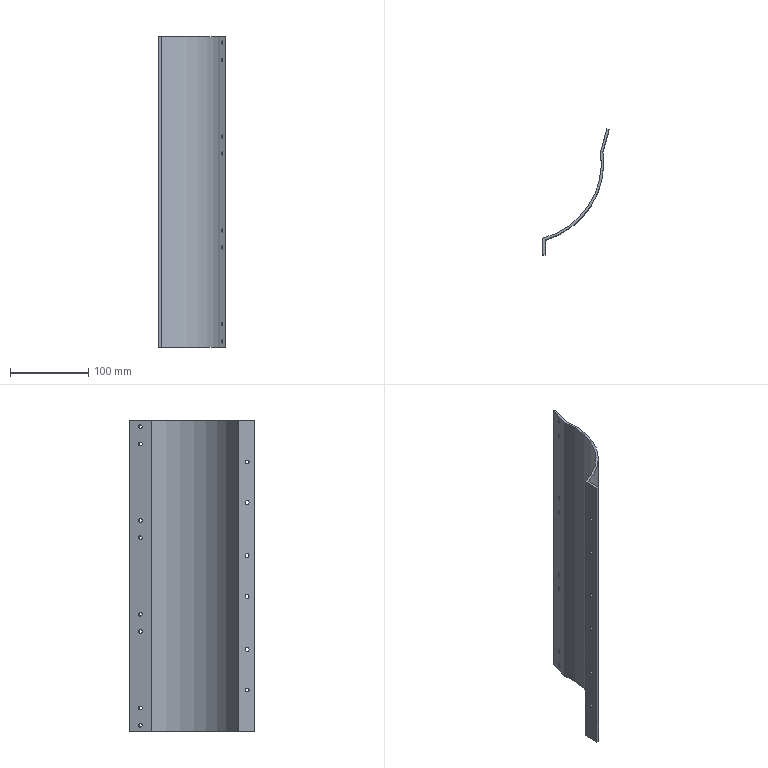Part | SolidWorks | features BaseBody 1 | 1 solid | 38 faces | box 85.064 x 161.136 x 398 mm | volume 233857 mm3 | cylinder 30 | plane 8 | commonest cylinder face diameters 5 x28 200 x1 206 x1
STEP:
#1=CARTESIAN_POINT('',(103.077,28.708,-32.5));
#2=VERTEX_POINT('',#1);
#3=CARTESIAN_POINT('',(103.077,28.708,-27.5));
#4=VERTEX_POINT('',#3);
#5=CARTESIAN_POINT('',(103.077,28.708,-30.));
#6=DIRECTION('',(0.9619,-0.2734,0.));
#7=DIRECTION('',(0.,0.,1.));
#8=AXIS2_PLACEMENT_3D('',#5,#6,#7);
#9=CIRCLE('',#8,2.5);
#10=EDGE_CURVE('',#2,#4,#9,.T.);
#11=ORIENTED_EDGE('',*,*,#10,.F.);
#12=CARTESIAN_POINT('',(105.962,27.888,-32.5));
#13=VERTEX_POINT('',#12);
#14=CARTESIAN_POINT('',(105.962,27.888,-32.5));
#15=DIRECTION('',(0.9619,-0.2734,0.));
#16=VECTOR('',#15,1000.);
#17=LINE('',#14,#16);
#18=EDGE_CURVE('',#2,#13,#17,.T.);
#19=ORIENTED_EDGE('',*,*,#18,.T.);
#20=CARTESIAN_POINT('',(105.962,27.888,-27.5));
#21=VERTEX_POINT('',#20);
#22=CARTESIAN_POINT('',(105.962,27.888,-30.));
#23=DIRECTION('',(-0.9619,0.2734,0.));
#24=DIRECTION('',(0.,0.,1.));
#25=AXIS2_PLACEMENT_3D('',#22,#23,#24);
#26=CIRCLE('',#25,2.5);
#27=EDGE_CURVE('',#21,#13,#26,.T.);
#28=ORIENTED_EDGE('',*,*,#27,.F.);
#29=CARTESIAN_POINT('',(105.962,27.888,-27.5));
#30=DIRECTION('',(0.9619,-0.2734,0.));
#31=VECTOR('',#30,1000.);
#32=LINE('',#29,#31);
#33=EDGE_CURVE('',#4,#21,#32,.T.);
#34=ORIENTED_EDGE('',*,*,#33,.F.);
#35=EDGE_LOOP('',(#11,#19,#28,#34));
#36=FACE_OUTER_BOUND('',#35,.T.);
#37=CARTESIAN_POINT('',(105.962,27.888,-30.));
#38=DIRECTION('',(0.9619,-0.2734,0.));
#39=DIRECTION('',(0.,0.,1.));
#40=AXIS2_PLACEMENT_3D('',#37,#38,#39);
#41=CYLINDRICAL_SURFACE('',#40,2.5);
#42=ADVANCED_FACE('',(#36),#41,.F.);
#43=CARTESIAN_POINT('',(103.077,28.708,-10.5));
#44=VERTEX_POINT('',#43);
#45=CARTESIAN_POINT('',(103.077,28.708,-5.5));
#46=VERTEX_POINT('',#45);
#47=CARTESIAN_POINT('',(103.077,28.708,-8.));
#48=DIRECTION('',(0.9619,-0.2734,0.));
#49=DIRECTION('',(0.,0.,1.));
#50=AXIS2_PLACEMENT_3D('',#47,#48,#49);
#51=CIRCLE('',#50,2.5);
#52=EDGE_CURVE('',#44,#46,#51,.T.);
#53=ORIENTED_EDGE('',*,*,#52,.F.);
#54=CARTESIAN_POINT('',(105.962,27.888,-10.5));
#55=VERTEX_POINT('',#54);
#56=CARTESIAN_POINT('',(105.962,27.888,-10.5));
#57=DIRECTION('',(0.9619,-0.2734,0.));
#58=VECTOR('',#57,1000.);
#59=LINE('',#56,#58);
#60=EDGE_CURVE('',#44,#55,#59,.T.);
#61=ORIENTED_EDGE('',*,*,#60,.T.);
#62=CARTESIAN_POINT('',(105.962,27.888,-5.5));
#63=VERTEX_POINT('',#62);
#64=CARTESIAN_POINT('',(105.962,27.888,-8.));
#65=DIRECTION('',(-0.9619,0.2734,0.));
#66=DIRECTION('',(0.,0.,1.));
#67=AXIS2_PLACEMENT_3D('',#64,#65,#66);
#68=CIRCLE('',#67,2.5);
#69=EDGE_CURVE('',#63,#55,#68,.T.);
#70=ORIENTED_EDGE('',*,*,#69,.F.);
#71=CARTESIAN_POINT('',(105.962,27.888,-5.5));
#72=DIRECTION('',(0.9619,-0.2734,0.));
#73=VECTOR('',#72,1000.);
#74=LINE('',#71,#73);
#75=EDGE_CURVE('',#46,#63,#74,.T.);
#76=ORIENTED_EDGE('',*,*,#75,.F.);
#77=EDGE_LOOP('',(#53,#61,#70,#76));
#78=FACE_OUTER_BOUND('',#77,.T.);
#79=CARTESIAN_POINT('',(105.962,27.888,-8.));
#80=DIRECTION('',(0.9619,-0.2734,0.));
#81=DIRECTION('',(0.,0.,1.));
#82=AXIS2_PLACEMENT_3D('',#79,#80,#81);
#83=CYLINDRICAL_SURFACE('',#82,2.5);
#84=ADVANCED_FACE('',(#78),#83,.F.);
#85=CARTESIAN_POINT('',(103.077,28.708,-152.5));
#86=VERTEX_POINT('',#85);
#87=CARTESIAN_POINT('',(103.077,28.708,-147.5));
#88=VERTEX_POINT('',#87);
#89=CARTESIAN_POINT('',(103.077,28.708,-150.));
#90=DIRECTION('',(0.9619,-0.2734,0.));
#91=DIRECTION('',(0.,0.,1.));
#92=AXIS2_PLACEMENT_3D('',#89,#90,#91);
#93=CIRCLE('',#92,2.5);
#94=EDGE_CURVE('',#86,#88,#93,.T.);
#95=ORIENTED_EDGE('',*,*,#94,.F.);
#96=CARTESIAN_POINT('',(105.962,27.888,-152.5));
#97=VERTEX_POINT('',#96);
#98=CARTESIAN_POINT('',(105.962,27.888,-152.5));
#99=DIRECTION('',(0.9619,-0.2734,0.));
#100=VECTOR('',#99,1000.);
#101=LINE('',#98,#100);
#102=EDGE_CURVE('',#86,#97,#101,.T.);
#103=ORIENTED_EDGE('',*,*,#102,.T.);
#104=CARTESIAN_POINT('',(105.962,27.888,-147.5));
#105=VERTEX_POINT('',#104);
#106=CARTESIAN_POINT('',(105.962,27.888,-150.));
#107=DIRECTION('',(-0.9619,0.2734,0.));
#108=DIRECTION('',(0.,0.,1.));
#109=AXIS2_PLACEMENT_3D('',#106,#107,#108);
#110=CIRCLE('',#109,2.5);
#111=EDGE_CURVE('',#105,#97,#110,.T.);
#112=ORIENTED_EDGE('',*,*,#111,.F.);
#113=CARTESIAN_POINT('',(105.962,27.888,-147.5));
#114=DIRECTION('',(0.9619,-0.2734,0.));
#115=VECTOR('',#114,1000.);
#116=LINE('',#113,#115);
#117=EDGE_CURVE('',#88,#105,#116,.T.);
#118=ORIENTED_EDGE('',*,*,#117,.F.);
#119=EDGE_LOOP('',(#95,#103,#112,#118));
#120=FACE_OUTER_BOUND('',#119,.T.);
#121=CARTESIAN_POINT('',(105.962,27.888,-150.));
#122=DIRECTION('',(0.9619,-0.2734,0.));
#123=DIRECTION('',(0.,0.,1.));
#124=AXIS2_PLACEMENT_3D('',#121,#122,#123);
#125=CYLINDRICAL_SURFACE('',#124,2.5);
#126=ADVANCED_FACE('',(#120),#125,.F.);
#127=CARTESIAN_POINT('',(103.077,28.708,-130.5));
#128=VERTEX_POINT('',#127);
#129=CARTESIAN_POINT('',(103.077,28.708,-125.5));
#130=VERTEX_POINT('',#129);
#131=CARTESIAN_POINT('',(103.077,28.708,-128.));
#132=DIRECTION('',(0.9619,-0.2734,0.));
#133=DIRECTION('',(0.,0.,1.));
#134=AXIS2_PLACEMENT_3D('',#131,#132,#133);
#135=CIRCLE('',#134,2.5);
#136=EDGE_CURVE('',#128,#130,#135,.T.);
#137=ORIENTED_EDGE('',*,*,#136,.F.);
#138=CARTESIAN_POINT('',(105.962,27.888,-130.5));
#139=VERTEX_POINT('',#138);
#140=CARTESIAN_POINT('',(105.962,27.888,-130.5));
#141=DIRECTION('',(0.9619,-0.2734,0.));
#142=VECTOR('',#141,1000.);
#143=LINE('',#140,#142);
#144=EDGE_CURVE('',#128,#139,#143,.T.);
#145=ORIENTED_EDGE('',*,*,#144,.T.);
#146=CARTESIAN_POINT('',(105.962,27.888,-125.5));
#147=VERTEX_POINT('',#146);
#148=CARTESIAN_POINT('',(105.962,27.888,-128.));
#149=DIRECTION('',(-0.9619,0.2734,0.));
#150=DIRECTION('',(0.,0.,1.));
#151=AXIS2_PLACEMENT_3D('',#148,#149,#150);
#152=CIRCLE('',#151,2.5);
#153=EDGE_CURVE('',#147,#139,#152,.T.);
#154=ORIENTED_EDGE('',*,*,#153,.F.);
#155=CARTESIAN_POINT('',(105.962,27.888,-125.5));
#156=DIRECTION('',(0.9619,-0.2734,0.));
#157=VECTOR('',#156,1000.);
#158=LINE('',#155,#157);
#159=EDGE_CURVE('',#130,#147,#158,.T.);
#160=ORIENTED_EDGE('',*,*,#159,.F.);
#161=EDGE_LOOP('',(#137,#145,#154,#160));
#162=FACE_OUTER_BOUND('',#161,.T.);
#163=CARTESIAN_POINT('',(105.962,27.888,-128.));
#164=DIRECTION('',(0.9619,-0.2734,0.));
#165=DIRECTION('',(0.,0.,1.));
#166=AXIS2_PLACEMENT_3D('',#163,#164,#165);
#167=CYLINDRICAL_SURFACE('',#166,2.5);
#168=ADVANCED_FACE('',(#162),#167,.F.);
#169=CARTESIAN_POINT('',(103.077,28.708,-272.5));
#170=VERTEX_POINT('',#169);
#171=CARTESIAN_POINT('',(103.077,28.708,-267.5));
#172=VERTEX_POINT('',#171);
#173=CARTESIAN_POINT('',(103.077,28.708,-270.));
#174=DIRECTION('',(0.9619,-0.2734,0.));
#175=DIRECTION('',(0.,0.,1.));
#176=AXIS2_PLACEMENT_3D('',#173,#174,#175);
#177=CIRCLE('',#176,2.5);
#178=EDGE_CURVE('',#170,#172,#177,.T.);
#179=ORIENTED_EDGE('',*,*,#178,.F.);
#180=CARTESIAN_POINT('',(105.962,27.888,-272.5));
#181=VERTEX_POINT('',#180);
#182=CARTESIAN_POINT('',(105.962,27.888,-272.5));
#183=DIRECTION('',(0.9619,-0.2734,0.));
#184=VECTOR('',#183,1000.);
#185=LINE('',#182,#184);
#186=EDGE_CURVE('',#170,#181,#185,.T.);
#187=ORIENTED_EDGE('',*,*,#186,.T.);
#188=CARTESIAN_POINT('',(105.962,27.888,-267.5));
#189=VERTEX_POINT('',#188);
#190=CARTESIAN_POINT('',(105.962,27.888,-270.));
#191=DIRECTION('',(-0.9619,0.2734,0.));
#192=DIRECTION('',(0.,0.,1.));
#193=AXIS2_PLACEMENT_3D('',#190,#191,#192);
#194=CIRCLE('',#193,2.5);
#195=EDGE_CURVE('',#189,#181,#194,.T.);
#196=ORIENTED_EDGE('',*,*,#195,.F.);
#197=CARTESIAN_POINT('',(105.962,27.888,-267.5));
#198=DIRECTION('',(0.9619,-0.2734,0.));
#199=VECTOR('',#198,1000.);
#200=LINE('',#197,#199);
#201=EDGE_CURVE('',#172,#189,#200,.T.);
#202=ORIENTED_EDGE('',*,*,#201,.F.);
#203=EDGE_LOOP('',(#179,#187,#196,#202));
#204=FACE_OUTER_BOUND('',#203,.T.);
#205=CARTESIAN_POINT('',(105.962,27.888,-270.));
#206=DIRECTION('',(0.9619,-0.2734,0.));
#207=DIRECTION('',(0.,0.,1.));
#208=AXIS2_PLACEMENT_3D('',#205,#206,#207);
#209=CYLINDRICAL_SURFACE('',#208,2.5);
#210=ADVANCED_FACE('',(#204),#209,.F.);
#211=CARTESIAN_POINT('',(103.077,28.708,-250.5));
#212=VERTEX_POINT('',#211);
#213=CARTESIAN_POINT('',(103.077,28.708,-245.5));
#214=VERTEX_POINT('',#213);
#215=CARTESIAN_POINT('',(103.077,28.708,-248.));
#216=DIRECTION('',(0.9619,-0.2734,0.));
#217=DIRECTION('',(0.,0.,1.));
#218=AXIS2_PLACEMENT_3D('',#215,#216,#217);
#219=CIRCLE('',#218,2.5);
#220=EDGE_CURVE('',#212,#214,#219,.T.);
#221=ORIENTED_EDGE('',*,*,#220,.F.);
#222=CARTESIAN_POINT('',(105.962,27.888,-250.5));
#223=VERTEX_POINT('',#222);
#224=CARTESIAN_POINT('',(105.962,27.888,-250.5));
#225=DIRECTION('',(0.9619,-0.2734,0.));
#226=VECTOR('',#225,1000.);
#227=LINE('',#224,#226);
#228=EDGE_CURVE('',#212,#223,#227,.T.);
#229=ORIENTED_EDGE('',*,*,#228,.T.);
#230=CARTESIAN_POINT('',(105.962,27.888,-245.5));
#231=VERTEX_POINT('',#230);
#232=CARTESIAN_POINT('',(105.962,27.888,-248.));
#233=DIRECTION('',(-0.9619,0.2734,0.));
#234=DIRECTION('',(0.,0.,1.));
#235=AXIS2_PLACEMENT_3D('',#232,#233,#234);
#236=CIRCLE('',#235,2.5);
#237=EDGE_CURVE('',#231,#223,#236,.T.);
#238=ORIENTED_EDGE('',*,*,#237,.F.);
#239=CARTESIAN_POINT('',(105.962,27.888,-245.5));
#240=DIRECTION('',(0.9619,-0.2734,0.));
#241=VECTOR('',#240,1000.);
#242=LINE('',#239,#241);
#243=EDGE_CURVE('',#214,#231,#242,.T.);
#244=ORIENTED_EDGE('',*,*,#243,.F.);
#245=EDGE_LOOP('',(#221,#229,#238,#244));
#246=FACE_OUTER_BOUND('',#245,.T.);
#247=CARTESIAN_POINT('',(105.962,27.888,-248.));
#248=DIRECTION('',(0.9619,-0.2734,0.));
#249=DIRECTION('',(0.,0.,1.));
#250=AXIS2_PLACEMENT_3D('',#247,#248,#249);
#251=CYLINDRICAL_SURFACE('',#250,2.5);
#252=ADVANCED_FACE('',(#246),#251,.F.);
#253=CARTESIAN_POINT('',(103.077,28.708,-392.5));
#254=VERTEX_POINT('',#253);
#255=CARTESIAN_POINT('',(103.077,28.708,-387.5));
#256=VERTEX_POINT('',#255);
#257=CARTESIAN_POINT('',(103.077,28.708,-390.));
#258=DIRECTION('',(0.9619,-0.2734,0.));
#259=DIRECTION('',(0.,0.,1.));
#260=AXIS2_PLACEMENT_3D('',#257,#258,#259);
#261=CIRCLE('',#260,2.5);
#262=EDGE_CURVE('',#254,#256,#261,.T.);
#263=ORIENTED_EDGE('',*,*,#262,.F.);
#264=CARTESIAN_POINT('',(105.962,27.888,-392.5));
#265=VERTEX_POINT('',#264);
#266=CARTESIAN_POINT('',(105.962,27.888,-392.5));
#267=DIRECTION('',(0.9619,-0.2734,0.));
#268=VECTOR('',#267,1000.);
#269=LINE('',#266,#268);
#270=EDGE_CURVE('',#254,#265,#269,.T.);
#271=ORIENTED_EDGE('',*,*,#270,.T.);
#272=CARTESIAN_POINT('',(105.962,27.888,-387.5));
#273=VERTEX_POINT('',#272);
#274=CARTESIAN_POINT('',(105.962,27.888,-390.));
#275=DIRECTION('',(-0.9619,0.2734,0.));
#276=DIRECTION('',(0.,0.,1.));
#277=AXIS2_PLACEMENT_3D('',#274,#275,#276);
#278=CIRCLE('',#277,2.5);
#279=EDGE_CURVE('',#273,#265,#278,.T.);
#280=ORIENTED_EDGE('',*,*,#279,.F.);
#281=CARTESIAN_POINT('',(105.962,27.888,-387.5));
#282=DIRECTION('',(0.9619,-0.2734,0.));
#283=VECTOR('',#282,1000.);
#284=LINE('',#281,#283);
#285=EDGE_CURVE('',#256,#273,#284,.T.);
#286=ORIENTED_EDGE('',*,*,#285,.F.);
#287=EDGE_LOOP('',(#263,#271,#280,#286));
#288=FACE_OUTER_BOUND('',#287,.T.);
#289=CARTESIAN_POINT('',(105.962,27.888,-390.));
#290=DIRECTION('',(0.9619,-0.2734,0.));
#291=DIRECTION('',(0.,0.,1.));
#292=AXIS2_PLACEMENT_3D('',#289,#290,#291);
#293=CYLINDRICAL_SURFACE('',#292,2.5);
#294=ADVANCED_FACE('',(#288),#293,.F.);
#295=CARTESIAN_POINT('',(103.077,28.708,-370.5));
#296=VERTEX_POINT('',#295);
#297=CARTESIAN_POINT('',(103.077,28.708,-365.5));
#298=VERTEX_POINT('',#297);
#299=CARTESIAN_POINT('',(103.077,28.708,-368.));
#300=DIRECTION('',(0.9619,-0.2734,0.));
#301=DIRECTION('',(0.,0.,1.));
#302=AXIS2_PLACEMENT_3D('',#299,#300,#301);
#303=CIRCLE('',#302,2.5);
#304=EDGE_CURVE('',#296,#298,#303,.T.);
#305=ORIENTED_EDGE('',*,*,#304,.F.);
#306=CARTESIAN_POINT('',(105.962,27.888,-370.5));
#307=VERTEX_POINT('',#306);
#308=CARTESIAN_POINT('',(105.962,27.888,-370.5));
#309=DIRECTION('',(0.9619,-0.2734,0.));
#310=VECTOR('',#309,1000.);
#311=LINE('',#308,#310);
#312=EDGE_CURVE('',#296,#307,#311,.T.);
#313=ORIENTED_EDGE('',*,*,#312,.T.);
#314=CARTESIAN_POINT('',(105.962,27.888,-365.5));
#315=VERTEX_POINT('',#314);
#316=CARTESIAN_POINT('',(105.962,27.888,-368.));
#317=DIRECTION('',(-0.9619,0.2734,0.));
#318=DIRECTION('',(0.,0.,1.));
#319=AXIS2_PLACEMENT_3D('',#316,#317,#318);
#320=CIRCLE('',#319,2.5);
#321=EDGE_CURVE('',#315,#307,#320,.T.);
#322=ORIENTED_EDGE('',*,*,#321,.F.);
#323=CARTESIAN_POINT('',(105.962,27.888,-365.5));
#324=DIRECTION('',(0.9619,-0.2734,0.));
#325=VECTOR('',#324,1000.);
#326=LINE('',#323,#325);
#327=EDGE_CURVE('',#298,#315,#326,.T.);
#328=ORIENTED_EDGE('',*,*,#327,.F.);
#329=EDGE_LOOP('',(#305,#313,#322,#328));
#330=FACE_OUTER_BOUND('',#329,.T.);
#331=CARTESIAN_POINT('',(105.962,27.888,-368.));
#332=DIRECTION('',(0.9619,-0.2734,0.));
#333=DIRECTION('',(0.,0.,1.));
#334=AXIS2_PLACEMENT_3D('',#331,#332,#333);
#335=CYLINDRICAL_SURFACE('',#334,2.5);
#336=ADVANCED_FACE('',(#330),#335,.F.);
#337=CARTESIAN_POINT('',(25.,-108.,-55.5));
#338=VERTEX_POINT('',#337);
#339=CARTESIAN_POINT('',(25.,-108.,-50.5));
#340=VERTEX_POINT('',#339);
#341=CARTESIAN_POINT('',(25.,-108.,-53.));
#342=DIRECTION('',(1.,0.,0.));
#343=DIRECTION('',(0.,0.,1.));
#344=AXIS2_PLACEMENT_3D('',#341,#342,#343);
#345=CIRCLE('',#344,2.5);
#346=EDGE_CURVE('',#338,#340,#345,.T.);
#347=ORIENTED_EDGE('',*,*,#346,.F.);
#348=CARTESIAN_POINT('',(28.,-108.,-55.5));
#349=VERTEX_POINT('',#348);
#350=CARTESIAN_POINT('',(28.,-108.,-55.5));
#351=DIRECTION('',(1.,0.,0.));
#352=VECTOR('',#351,1000.);
#353=LINE('',#350,#352);
#354=EDGE_CURVE('',#338,#349,#353,.T.);
#355=ORIENTED_EDGE('',*,*,#354,.T.);
#356=CARTESIAN_POINT('',(28.,-108.,-50.5));
#357=VERTEX_POINT('',#356);
#358=CARTESIAN_POINT('',(28.,-108.,-53.));
#359=DIRECTION('',(-1.,0.,0.));
#360=DIRECTION('',(0.,0.,1.));
#361=AXIS2_PLACEMENT_3D('',#358,#359,#360);
#362=CIRCLE('',#361,2.5);
#363=EDGE_CURVE('',#357,#349,#362,.T.);
#364=ORIENTED_EDGE('',*,*,#363,.F.);
#365=CARTESIAN_POINT('',(28.,-108.,-50.5));
#366=DIRECTION('',(1.,0.,0.));
#367=VECTOR('',#366,1000.);
#368=LINE('',#365,#367);
#369=EDGE_CURVE('',#340,#357,#368,.T.);
#370=ORIENTED_EDGE('',*,*,#369,.F.);
#371=EDGE_LOOP('',(#347,#355,#364,#370));
#372=FACE_OUTER_BOUND('',#371,.T.);
#373=CARTESIAN_POINT('',(28.,-108.,-53.));
#374=DIRECTION('',(1.,0.,0.));
#375=DIRECTION('',(0.,0.,1.));
#376=AXIS2_PLACEMENT_3D('',#373,#374,#375);
#377=CYLINDRICAL_SURFACE('',#376,2.5);
#378=ADVANCED_FACE('',(#372),#377,.F.);
#379=CARTESIAN_POINT('',(25.,-108.,-107.5));
#380=VERTEX_POINT('',#379);
#381=CARTESIAN_POINT('',(25.,-108.,-102.5));
#382=VERTEX_POINT('',#381);
#383=CARTESIAN_POINT('',(25.,-108.,-105.));
#384=DIRECTION('',(1.,0.,0.));
#385=DIRECTION('',(0.,0.,1.));
#386=AXIS2_PLACEMENT_3D('',#383,#384,#385);
#387=CIRCLE('',#386,2.5);
#388=EDGE_CURVE('',#380,#382,#387,.T.);
#389=ORIENTED_EDGE('',*,*,#388,.F.);
#390=CARTESIAN_POINT('',(28.,-108.,-107.5));
#391=VERTEX_POINT('',#390);
#392=CARTESIAN_POINT('',(28.,-108.,-107.5));
#393=DIRECTION('',(1.,0.,0.));
#394=VECTOR('',#393,1000.);
#395=LINE('',#392,#394);
#396=EDGE_CURVE('',#380,#391,#395,.T.);
#397=ORIENTED_EDGE('',*,*,#396,.T.);
#398=CARTESIAN_POINT('',(28.,-108.,-102.5));
#399=VERTEX_POINT('',#398);
#400=CARTESIAN_POINT('',(28.,-108.,-105.));
#401=DIRECTION('',(-1.,0.,0.));
#402=DIRECTION('',(0.,0.,1.));
#403=AXIS2_PLACEMENT_3D('',#400,#401,#402);
#404=CIRCLE('',#403,2.5);
#405=EDGE_CURVE('',#399,#391,#404,.T.);
#406=ORIENTED_EDGE('',*,*,#405,.F.);
#407=CARTESIAN_POINT('',(28.,-108.,-102.5));
#408=DIRECTION('',(1.,0.,0.));
#409=VECTOR('',#408,1000.);
#410=LINE('',#407,#409);
#411=EDGE_CURVE('',#382,#399,#410,.T.);
#412=ORIENTED_EDGE('',*,*,#411,.F.);
#413=EDGE_LOOP('',(#389,#397,#406,#412));
#414=FACE_OUTER_BOUND('',#413,.T.);
#415=CARTESIAN_POINT('',(28.,-108.,-105.));
#416=DIRECTION('',(1.,0.,0.));
#417=DIRECTION('',(0.,0.,1.));
#418=AXIS2_PLACEMENT_3D('',#415,#416,#417);
#419=CYLINDRICAL_SURFACE('',#418,2.5);
#420=ADVANCED_FACE('',(#414),#419,.F.);
#421=CARTESIAN_POINT('',(25.,-108.,-175.5));
#422=VERTEX_POINT('',#421);
#423=CARTESIAN_POINT('',(25.,-108.,-170.5));
#424=VERTEX_POINT('',#423);
#425=CARTESIAN_POINT('',(25.,-108.,-173.));
#426=DIRECTION('',(1.,0.,0.));
#427=DIRECTION('',(0.,0.,1.));
#428=AXIS2_PLACEMENT_3D('',#425,#426,#427);
#429=CIRCLE('',#428,2.5);
#430=EDGE_CURVE('',#422,#424,#429,.T.);
#431=ORIENTED_EDGE('',*,*,#430,.F.);
#432=CARTESIAN_POINT('',(28.,-108.,-175.5));
#433=VERTEX_POINT('',#432);
#434=CARTESIAN_POINT('',(28.,-108.,-175.5));
#435=DIRECTION('',(1.,0.,0.));
#436=VECTOR('',#435,1000.);
#437=LINE('',#434,#436);
#438=EDGE_CURVE('',#422,#433,#437,.T.);
#439=ORIENTED_EDGE('',*,*,#438,.T.);
#440=CARTESIAN_POINT('',(28.,-108.,-170.5));
#441=VERTEX_POINT('',#440);
#442=CARTESIAN_POINT('',(28.,-108.,-173.));
#443=DIRECTION('',(-1.,0.,0.));
#444=DIRECTION('',(0.,0.,1.));
#445=AXIS2_PLACEMENT_3D('',#442,#443,#444);
#446=CIRCLE('',#445,2.5);
#447=EDGE_CURVE('',#441,#433,#446,.T.);
#448=ORIENTED_EDGE('',*,*,#447,.F.);
#449=CARTESIAN_POINT('',(28.,-108.,-170.5));
#450=DIRECTION('',(1.,0.,0.));
#451=VECTOR('',#450,1000.);
#452=LINE('',#449,#451);
#453=EDGE_CURVE('',#424,#441,#452,.T.);
#454=ORIENTED_EDGE('',*,*,#453,.F.);
#455=EDGE_LOOP('',(#431,#439,#448,#454));
#456=FACE_OUTER_BOUND('',#455,.T.);
#457=CARTESIAN_POINT('',(28.,-108.,-173.));
#458=DIRECTION('',(1.,0.,0.));
#459=DIRECTION('',(0.,0.,1.));
#460=AXIS2_PLACEMENT_3D('',#457,#458,#459);
#461=CYLINDRICAL_SURFACE('',#460,2.5);
#462=ADVANCED_FACE('',(#456),#461,.F.);
#463=CARTESIAN_POINT('',(25.,-108.,-227.5));
#464=VERTEX_POINT('',#463);
#465=CARTESIAN_POINT('',(25.,-108.,-222.5));
#466=VERTEX_POINT('',#465);
#467=CARTESIAN_POINT('',(25.,-108.,-225.));
#468=DIRECTION('',(1.,0.,0.));
#469=DIRECTION('',(0.,0.,1.));
#470=AXIS2_PLACEMENT_3D('',#467,#468,#469);
#471=CIRCLE('',#470,2.5);
#472=EDGE_CURVE('',#464,#466,#471,.T.);
#473=ORIENTED_EDGE('',*,*,#472,.F.);
#474=CARTESIAN_POINT('',(28.,-108.,-227.5));
#475=VERTEX_POINT('',#474);
#476=CARTESIAN_POINT('',(28.,-108.,-227.5));
#477=DIRECTION('',(1.,0.,0.));
#478=VECTOR('',#477,1000.);
#479=LINE('',#476,#478);
#480=EDGE_CURVE('',#464,#475,#479,.T.);
#481=ORIENTED_EDGE('',*,*,#480,.T.);
#482=CARTESIAN_POINT('',(28.,-108.,-222.5));
#483=VERTEX_POINT('',#482);
#484=CARTESIAN_POINT('',(28.,-108.,-225.));
#485=DIRECTION('',(-1.,0.,0.));
#486=DIRECTION('',(0.,0.,1.));
#487=AXIS2_PLACEMENT_3D('',#484,#485,#486);
#488=CIRCLE('',#487,2.5);
#489=EDGE_CURVE('',#483,#475,#488,.T.);
#490=ORIENTED_EDGE('',*,*,#489,.F.);
#491=CARTESIAN_POINT('',(28.,-108.,-222.5));
#492=DIRECTION('',(1.,0.,0.));
#493=VECTOR('',#492,1000.);
#494=LINE('',#491,#493);
#495=EDGE_CURVE('',#466,#483,#494,.T.);
#496=ORIENTED_EDGE('',*,*,#495,.F.);
#497=EDGE_LOOP('',(#473,#481,#490,#496));
#498=FACE_OUTER_BOUND('',#497,.T.);
#499=CARTESIAN_POINT('',(28.,-108.,-225.));
#500=DIRECTION('',(1.,0.,0.));
#501=DIRECTION('',(0.,0.,1.));
#502=AXIS2_PLACEMENT_3D('',#499,#500,#501);
#503=CYLINDRICAL_SURFACE('',#502,2.5);
#504=ADVANCED_FACE('',(#498),#503,.F.);
#505=CARTESIAN_POINT('',(25.,-108.,-295.5));
#506=VERTEX_POINT('',#505);
#507=CARTESIAN_POINT('',(25.,-108.,-290.5));
#508=VERTEX_POINT('',#507);
#509=CARTESIAN_POINT('',(25.,-108.,-293.));
#510=DIRECTION('',(1.,0.,0.));
#511=DIRECTION('',(0.,0.,1.));
#512=AXIS2_PLACEMENT_3D('',#509,#510,#511);
#513=CIRCLE('',#512,2.5);
#514=EDGE_CURVE('',#506,#508,#513,.T.);
#515=ORIENTED_EDGE('',*,*,#514,.F.);
#516=CARTESIAN_POINT('',(28.,-108.,-295.5));
#517=VERTEX_POINT('',#516);
#518=CARTESIAN_POINT('',(28.,-108.,-295.5));
#519=DIRECTION('',(1.,0.,0.));
#520=VECTOR('',#519,1000.);
#521=LINE('',#518,#520);
#522=EDGE_CURVE('',#506,#517,#521,.T.);
#523=ORIENTED_EDGE('',*,*,#522,.T.);
#524=CARTESIAN_POINT('',(28.,-108.,-290.5));
#525=VERTEX_POINT('',#524);
#526=CARTESIAN_POINT('',(28.,-108.,-293.));
#527=DIRECTION('',(-1.,0.,0.));
#528=DIRECTION('',(0.,0.,1.));
#529=AXIS2_PLACEMENT_3D('',#526,#527,#528);
#530=CIRCLE('',#529,2.5);
#531=EDGE_CURVE('',#525,#517,#530,.T.);
#532=ORIENTED_EDGE('',*,*,#531,.F.);
#533=CARTESIAN_POINT('',(28.,-108.,-290.5));
#534=DIRECTION('',(1.,0.,0.));
#535=VECTOR('',#534,1000.);
#536=LINE('',#533,#535);
#537=EDGE_CURVE('',#508,#525,#536,.T.);
#538=ORIENTED_EDGE('',*,*,#537,.F.);
#539=EDGE_LOOP('',(#515,#523,#532,#538));
#540=FACE_OUTER_BOUND('',#539,.T.);
#541=CARTESIAN_POINT('',(28.,-108.,-293.));
#542=DIRECTION('',(1.,0.,0.));
#543=DIRECTION('',(0.,0.,1.));
#544=AXIS2_PLACEMENT_3D('',#541,#542,#543);
#545=CYLINDRICAL_SURFACE('',#544,2.5);
#546=ADVANCED_FACE('',(#540),#545,.F.);
#547=CARTESIAN_POINT('',(25.,-108.,-347.5));
#548=VERTEX_POINT('',#547);
#549=CARTESIAN_POINT('',(25.,-108.,-342.5));
#550=VERTEX_POINT('',#549);
#551=CARTESIAN_POINT('',(25.,-108.,-345.));
#552=DIRECTION('',(1.,0.,0.));
#553=DIRECTION('',(0.,0.,1.));
#554=AXIS2_PLACEMENT_3D('',#551,#552,#553);
#555=CIRCLE('',#554,2.5);
#556=EDGE_CURVE('',#548,#550,#555,.T.);
#557=ORIENTED_EDGE('',*,*,#556,.F.);
#558=CARTESIAN_POINT('',(28.,-108.,-347.5));
#559=VERTEX_POINT('',#558);
#560=CARTESIAN_POINT('',(28.,-108.,-347.5));
#561=DIRECTION('',(1.,0.,0.));
#562=VECTOR('',#561,1000.);
#563=LINE('',#560,#562);
#564=EDGE_CURVE('',#548,#559,#563,.T.);
#565=ORIENTED_EDGE('',*,*,#564,.T.);
#566=CARTESIAN_POINT('',(28.,-108.,-342.5));
#567=VERTEX_POINT('',#566);
#568=CARTESIAN_POINT('',(28.,-108.,-345.));
#569=DIRECTION('',(-1.,0.,0.));
#570=DIRECTION('',(0.,0.,1.));
#571=AXIS2_PLACEMENT_3D('',#568,#569,#570);
#572=CIRCLE('',#571,2.5);
#573=EDGE_CURVE('',#567,#559,#572,.T.);
#574=ORIENTED_EDGE('',*,*,#573,.F.);
#575=CARTESIAN_POINT('',(28.,-108.,-342.5));
#576=DIRECTION('',(1.,0.,0.));
#577=VECTOR('',#576,1000.);
#578=LINE('',#575,#577);
#579=EDGE_CURVE('',#550,#567,#578,.T.);
#580=ORIENTED_EDGE('',*,*,#579,.F.);
#581=EDGE_LOOP('',(#557,#565,#574,#580));
#582=FACE_OUTER_BOUND('',#581,.T.);
#583=CARTESIAN_POINT('',(28.,-108.,-345.));
#584=DIRECTION('',(1.,0.,0.));
#585=DIRECTION('',(0.,0.,1.));
#586=AXIS2_PLACEMENT_3D('',#583,#584,#585);
#587=CYLINDRICAL_SURFACE('',#586,2.5);
#588=ADVANCED_FACE('',(#582),#587,.F.);
#589=ORIENTED_EDGE('',*,*,#363,.T.);
#590=CARTESIAN_POINT('',(28.,-108.,-53.));
#591=DIRECTION('',(-1.,0.,0.));
#592=DIRECTION('',(0.,0.,1.));
#593=AXIS2_PLACEMENT_3D('',#590,#591,#592);
#594=CIRCLE('',#593,2.5);
#595=EDGE_CURVE('',#349,#357,#594,.T.);
#596=ORIENTED_EDGE('',*,*,#595,.T.);
#597=EDGE_LOOP('',(#589,#596));
#598=FACE_BOUND('',#597,.T.);
#599=ORIENTED_EDGE('',*,*,#405,.T.);
#600=CARTESIAN_POINT('',(28.,-108.,-105.));
#601=DIRECTION('',(-1.,0.,0.));
#602=DIRECTION('',(0.,0.,1.));
#603=AXIS2_PLACEMENT_3D('',#600,#601,#602);
#604=CIRCLE('',#603,2.5);
#605=EDGE_CURVE('',#391,#399,#604,.T.);
#606=ORIENTED_EDGE('',*,*,#605,.T.);
#607=EDGE_LOOP('',(#599,#606));
#608=FACE_BOUND('',#607,.T.);
#609=ORIENTED_EDGE('',*,*,#447,.T.);
#610=CARTESIAN_POINT('',(28.,-108.,-173.));
#611=DIRECTION('',(-1.,0.,0.));
#612=DIRECTION('',(0.,0.,1.));
#613=AXIS2_PLACEMENT_3D('',#610,#611,#612);
#614=CIRCLE('',#613,2.5);
#615=EDGE_CURVE('',#433,#441,#614,.T.);
#616=ORIENTED_EDGE('',*,*,#615,.T.);
#617=EDGE_LOOP('',(#609,#616));
#618=FACE_BOUND('',#617,.T.);
#619=ORIENTED_EDGE('',*,*,#489,.T.);
#620=CARTESIAN_POINT('',(28.,-108.,-225.));
#621=DIRECTION('',(-1.,0.,0.));
#622=DIRECTION('',(0.,0.,1.));
#623=AXIS2_PLACEMENT_3D('',#620,#621,#622);
#624=CIRCLE('',#623,2.5);
#625=EDGE_CURVE('',#475,#483,#624,.T.);
#626=ORIENTED_EDGE('',*,*,#625,.T.);
#627=EDGE_LOOP('',(#619,#626));
#628=FACE_BOUND('',#627,.T.);
#629=ORIENTED_EDGE('',*,*,#531,.T.);
#630=CARTESIAN_POINT('',(28.,-108.,-293.));
#631=DIRECTION('',(-1.,0.,0.));
#632=DIRECTION('',(0.,0.,1.));
#633=AXIS2_PLACEMENT_3D('',#630,#631,#632);
#634=CIRCLE('',#633,2.5);
#635=EDGE_CURVE('',#517,#525,#634,.T.);
#636=ORIENTED_EDGE('',*,*,#635,.T.);
#637=EDGE_LOOP('',(#629,#636));
#638=FACE_BOUND('',#637,.T.);
#639=ORIENTED_EDGE('',*,*,#573,.T.);
#640=CARTESIAN_POINT('',(28.,-108.,-345.));
#641=DIRECTION('',(-1.,0.,0.));
#642=DIRECTION('',(0.,0.,1.));
#643=AXIS2_PLACEMENT_3D('',#640,#641,#642);
#644=CIRCLE('',#643,2.5);
#645=EDGE_CURVE('',#559,#567,#644,.T.);
#646=ORIENTED_EDGE('',*,*,#645,.T.);
#647=EDGE_LOOP('',(#639,#646));
#648=FACE_BOUND('',#647,.T.);
#649=CARTESIAN_POINT('',(28.,-118.,0.));
#650=VERTEX_POINT('',#649);
#651=CARTESIAN_POINT('',(28.,-99.121,0.));
#652=VERTEX_POINT('',#651);
#653=CARTESIAN_POINT('',(28.,-118.,0.));
#654=DIRECTION('',(0.,1.,0.));
#655=VECTOR('',#654,1000.);
#656=LINE('',#653,#655);
#657=EDGE_CURVE('',#650,#652,#656,.T.);
#658=ORIENTED_EDGE('',*,*,#657,.F.);
#659=CARTESIAN_POINT('',(28.,-118.,-398.));
#660=VERTEX_POINT('',#659);
#661=CARTESIAN_POINT('',(28.,-118.,0.));
#662=DIRECTION('',(0.,0.,-1.));
#663=VECTOR('',#662,1000.);
#664=LINE('',#661,#663);
#665=EDGE_CURVE('',#650,#660,#664,.T.);
#666=ORIENTED_EDGE('',*,*,#665,.T.);
#667=CARTESIAN_POINT('',(28.,-99.121,-398.));
#668=VERTEX_POINT('',#667);
#669=CARTESIAN_POINT('',(28.,-118.,-398.));
#670=DIRECTION('',(0.,-1.,0.));
#671=VECTOR('',#670,1000.);
#672=LINE('',#669,#671);
#673=EDGE_CURVE('',#668,#660,#672,.T.);
#674=ORIENTED_EDGE('',*,*,#673,.F.);
#675=CARTESIAN_POINT('',(28.,-99.121,0.));
#676=DIRECTION('',(0.,0.,-1.));
#677=VECTOR('',#676,1000.);
#678=LINE('',#675,#677);
#679=EDGE_CURVE('',#652,#668,#678,.T.);
#680=ORIENTED_EDGE('',*,*,#679,.F.);
#681=EDGE_LOOP('',(#658,#666,#674,#680));
#682=FACE_OUTER_BOUND('',#681,.T.);
#683=CARTESIAN_POINT('',(28.,-99.121,0.));
#684=DIRECTION('',(1.,0.,0.));
#685=DIRECTION('',(0.,1.,0.));
#686=AXIS2_PLACEMENT_3D('',#683,#684,#685);
#687=PLANE('',#686);
#688=ADVANCED_FACE('',(#598,#608,#618,#628,#638,#648,#682),#687,.T.);
#689=CARTESIAN_POINT('',(102.034,14.07,0.));
#690=VERTEX_POINT('',#689);
#691=CARTESIAN_POINT('',(0.,0.,0.));
#692=DIRECTION('',(0.,0.,1.));
#693=DIRECTION('',(0.2718,-0.9623,0.));
#694=AXIS2_PLACEMENT_3D('',#691,#692,#693);
#695=CIRCLE('',#694,103.);
#696=EDGE_CURVE('',#652,#690,#695,.T.);
#697=ORIENTED_EDGE('',*,*,#696,.F.);
#698=ORIENTED_EDGE('',*,*,#679,.T.);
#699=CARTESIAN_POINT('',(102.034,14.07,-398.));
#700=VERTEX_POINT('',#699);
#701=CARTESIAN_POINT('',(0.,0.,-398.));
#702=DIRECTION('',(0.,0.,-1.));
#703=DIRECTION('',(0.2718,-0.9623,0.));
#704=AXIS2_PLACEMENT_3D('',#701,#702,#703);
#705=CIRCLE('',#704,103.);
#706=EDGE_CURVE('',#700,#668,#705,.T.);
#707=ORIENTED_EDGE('',*,*,#706,.F.);
#708=CARTESIAN_POINT('',(102.034,14.07,0.));
#709=DIRECTION('',(0.,0.,-1.));
#710=VECTOR('',#709,1000.);
#711=LINE('',#708,#710);
#712=EDGE_CURVE('',#690,#700,#711,.T.);
#713=ORIENTED_EDGE('',*,*,#712,.F.);
#714=EDGE_LOOP('',(#697,#698,#707,#713));
#715=FACE_OUTER_BOUND('',#714,.T.);
#716=CARTESIAN_POINT('',(0.,0.,0.));
#717=DIRECTION('',(0.,0.,1.));
#718=DIRECTION('',(0.2718,-0.9623,0.));
#719=AXIS2_PLACEMENT_3D('',#716,#717,#718);
#720=CYLINDRICAL_SURFACE('',#719,103.);
#721=ADVANCED_FACE('',(#715),#720,.T.);
#722=ORIENTED_EDGE('',*,*,#27,.T.);
#723=CARTESIAN_POINT('',(105.962,27.888,-30.));
#724=DIRECTION('',(-0.9619,0.2734,0.));
#725=DIRECTION('',(0.,0.,1.));
#726=AXIS2_PLACEMENT_3D('',#723,#724,#725);
#727=CIRCLE('',#726,2.5);
#728=EDGE_CURVE('',#13,#21,#727,.T.);
#729=ORIENTED_EDGE('',*,*,#728,.T.);
#730=EDGE_LOOP('',(#722,#729));
#731=FACE_BOUND('',#730,.T.);
#732=ORIENTED_EDGE('',*,*,#69,.T.);
#733=CARTESIAN_POINT('',(105.962,27.888,-8.));
#734=DIRECTION('',(-0.9619,0.2734,0.));
#735=DIRECTION('',(0.,0.,1.));
#736=AXIS2_PLACEMENT_3D('',#733,#734,#735);
#737=CIRCLE('',#736,2.5);
#738=EDGE_CURVE('',#55,#63,#737,.T.);
#739=ORIENTED_EDGE('',*,*,#738,.T.);
#740=EDGE_LOOP('',(#732,#739));
#741=FACE_BOUND('',#740,.T.);
#742=ORIENTED_EDGE('',*,*,#111,.T.);
#743=CARTESIAN_POINT('',(105.962,27.888,-150.));
#744=DIRECTION('',(-0.9619,0.2734,0.));
#745=DIRECTION('',(0.,0.,1.));
#746=AXIS2_PLACEMENT_3D('',#743,#744,#745);
#747=CIRCLE('',#746,2.5);
#748=EDGE_CURVE('',#97,#105,#747,.T.);
#749=ORIENTED_EDGE('',*,*,#748,.T.);
#750=EDGE_LOOP('',(#742,#749));
#751=FACE_BOUND('',#750,.T.);
#752=ORIENTED_EDGE('',*,*,#153,.T.);
#753=CARTESIAN_POINT('',(105.962,27.888,-128.));
#754=DIRECTION('',(-0.9619,0.2734,0.));
#755=DIRECTION('',(0.,0.,1.));
#756=AXIS2_PLACEMENT_3D('',#753,#754,#755);
#757=CIRCLE('',#756,2.5);
#758=EDGE_CURVE('',#139,#147,#757,.T.);
#759=ORIENTED_EDGE('',*,*,#758,.T.);
#760=EDGE_LOOP('',(#752,#759));
#761=FACE_BOUND('',#760,.T.);
#762=ORIENTED_EDGE('',*,*,#195,.T.);
#763=CARTESIAN_POINT('',(105.962,27.888,-270.));
#764=DIRECTION('',(-0.9619,0.2734,0.));
#765=DIRECTION('',(0.,0.,1.));
#766=AXIS2_PLACEMENT_3D('',#763,#764,#765);
#767=CIRCLE('',#766,2.5);
#768=EDGE_CURVE('',#181,#189,#767,.T.);
#769=ORIENTED_EDGE('',*,*,#768,.T.);
#770=EDGE_LOOP('',(#762,#769));
#771=FACE_BOUND('',#770,.T.);
#772=ORIENTED_EDGE('',*,*,#237,.T.);
#773=CARTESIAN_POINT('',(105.962,27.888,-248.));
#774=DIRECTION('',(-0.9619,0.2734,0.));
#775=DIRECTION('',(0.,0.,1.));
#776=AXIS2_PLACEMENT_3D('',#773,#774,#775);
#777=CIRCLE('',#776,2.5);
#778=EDGE_CURVE('',#223,#231,#777,.T.);
#779=ORIENTED_EDGE('',*,*,#778,.T.);
#780=EDGE_LOOP('',(#772,#779));
#781=FACE_BOUND('',#780,.T.);
#782=ORIENTED_EDGE('',*,*,#279,.T.);
#783=CARTESIAN_POINT('',(105.962,27.888,-390.));
#784=DIRECTION('',(-0.9619,0.2734,0.));
#785=DIRECTION('',(0.,0.,1.));
#786=AXIS2_PLACEMENT_3D('',#783,#784,#785);
#787=CIRCLE('',#786,2.5);
#788=EDGE_CURVE('',#265,#273,#787,.T.);
#789=ORIENTED_EDGE('',*,*,#788,.T.);
#790=EDGE_LOOP('',(#782,#789));
#791=FACE_BOUND('',#790,.T.);
#792=ORIENTED_EDGE('',*,*,#321,.T.);
#793=CARTESIAN_POINT('',(105.962,27.888,-368.));
#794=DIRECTION('',(-0.9619,0.2734,0.));
#795=DIRECTION('',(0.,0.,1.));
#796=AXIS2_PLACEMENT_3D('',#793,#794,#795);
#797=CIRCLE('',#796,2.5);
#798=EDGE_CURVE('',#307,#315,#797,.T.);
#799=ORIENTED_EDGE('',*,*,#798,.T.);
#800=EDGE_LOOP('',(#792,#799));
#801=FACE_BOUND('',#800,.T.);
#802=CARTESIAN_POINT('',(110.064,42.316,0.));
#803=VERTEX_POINT('',#802);
#804=CARTESIAN_POINT('',(102.034,14.07,0.));
#805=DIRECTION('',(0.2734,0.9619,0.));
#806=VECTOR('',#805,1000.);
#807=LINE('',#804,#806);
#808=EDGE_CURVE('',#690,#803,#807,.T.);
#809=ORIENTED_EDGE('',*,*,#808,.F.);
#810=ORIENTED_EDGE('',*,*,#712,.T.);
#811=CARTESIAN_POINT('',(110.064,42.316,-398.));
#812=VERTEX_POINT('',#811);
#813=CARTESIAN_POINT('',(102.034,14.07,-398.));
#814=DIRECTION('',(-0.2734,-0.9619,0.));
#815=VECTOR('',#814,1000.);
#816=LINE('',#813,#815);
#817=EDGE_CURVE('',#812,#700,#816,.T.);
#818=ORIENTED_EDGE('',*,*,#817,.F.);
#819=CARTESIAN_POINT('',(110.064,42.316,0.));
#820=DIRECTION('',(0.,0.,-1.));
#821=VECTOR('',#820,1000.);
#822=LINE('',#819,#821);
#823=EDGE_CURVE('',#803,#812,#822,.T.);
#824=ORIENTED_EDGE('',*,*,#823,.F.);
#825=EDGE_LOOP('',(#809,#810,#818,#824));
#826=FACE_OUTER_BOUND('',#825,.T.);
#827=CARTESIAN_POINT('',(110.064,42.316,0.));
#828=DIRECTION('',(0.9619,-0.2734,0.));
#829=DIRECTION('',(0.,0.,-1.));
#830=AXIS2_PLACEMENT_3D('',#827,#828,#829);
#831=PLANE('',#830);
#832=ADVANCED_FACE('',(#731,#741,#751,#761,#771,#781,#791,#801,#826),#831,.T.);
#833=CARTESIAN_POINT('',(107.178,43.136,0.));
#834=VERTEX_POINT('',#833);
#835=CARTESIAN_POINT('',(110.064,42.316,0.));
#836=DIRECTION('',(-0.9619,0.2734,0.));
#837=VECTOR('',#836,1000.);
#838=LINE('',#835,#837);
#839=EDGE_CURVE('',#803,#834,#838,.T.);
#840=ORIENTED_EDGE('',*,*,#839,.F.);
#841=ORIENTED_EDGE('',*,*,#823,.T.);
#842=CARTESIAN_POINT('',(107.178,43.136,-398.));
#843=VERTEX_POINT('',#842);
#844=CARTESIAN_POINT('',(110.064,42.316,-398.));
#845=DIRECTION('',(0.9619,-0.2734,0.));
#846=VECTOR('',#845,1000.);
#847=LINE('',#844,#846);
#848=EDGE_CURVE('',#843,#812,#847,.T.);
#849=ORIENTED_EDGE('',*,*,#848,.F.);
#850=CARTESIAN_POINT('',(107.178,43.136,0.));
#851=DIRECTION('',(0.,0.,-1.));
#852=VECTOR('',#851,1000.);
#853=LINE('',#850,#852);
#854=EDGE_CURVE('',#834,#843,#853,.T.);
#855=ORIENTED_EDGE('',*,*,#854,.F.);
#856=EDGE_LOOP('',(#840,#841,#849,#855));
#857=FACE_OUTER_BOUND('',#856,.T.);
#858=CARTESIAN_POINT('',(107.178,43.136,0.));
#859=DIRECTION('',(0.2734,0.9619,0.));
#860=DIRECTION('',(0.,0.,-1.));
#861=AXIS2_PLACEMENT_3D('',#858,#859,#860);
#862=PLANE('',#861);
#863=ADVANCED_FACE('',(#857),#862,.T.);
#864=CARTESIAN_POINT('',(103.077,28.708,-30.));
#865=DIRECTION('',(0.9619,-0.2734,0.));
#866=DIRECTION('',(0.,0.,1.));
#867=AXIS2_PLACEMENT_3D('',#864,#865,#866);
#868=CIRCLE('',#867,2.5);
#869=EDGE_CURVE('',#4,#2,#868,.T.);
#870=ORIENTED_EDGE('',*,*,#869,.T.);
#871=ORIENTED_EDGE('',*,*,#10,.T.);
#872=EDGE_LOOP('',(#870,#871));
#873=FACE_BOUND('',#872,.T.);
#874=CARTESIAN_POINT('',(103.077,28.708,-8.));
#875=DIRECTION('',(0.9619,-0.2734,0.));
#876=DIRECTION('',(0.,0.,1.));
#877=AXIS2_PLACEMENT_3D('',#874,#875,#876);
#878=CIRCLE('',#877,2.5);
#879=EDGE_CURVE('',#46,#44,#878,.T.);
#880=ORIENTED_EDGE('',*,*,#879,.T.);
#881=ORIENTED_EDGE('',*,*,#52,.T.);
#882=EDGE_LOOP('',(#880,#881));
#883=FACE_BOUND('',#882,.T.);
#884=CARTESIAN_POINT('',(103.077,28.708,-150.));
#885=DIRECTION('',(0.9619,-0.2734,0.));
#886=DIRECTION('',(0.,0.,1.));
#887=AXIS2_PLACEMENT_3D('',#884,#885,#886);
#888=CIRCLE('',#887,2.5);
#889=EDGE_CURVE('',#88,#86,#888,.T.);
#890=ORIENTED_EDGE('',*,*,#889,.T.);
#891=ORIENTED_EDGE('',*,*,#94,.T.);
#892=EDGE_LOOP('',(#890,#891));
#893=FACE_BOUND('',#892,.T.);
#894=CARTESIAN_POINT('',(103.077,28.708,-128.));
#895=DIRECTION('',(0.9619,-0.2734,0.));
#896=DIRECTION('',(0.,0.,1.));
#897=AXIS2_PLACEMENT_3D('',#894,#895,#896);
#898=CIRCLE('',#897,2.5);
#899=EDGE_CURVE('',#130,#128,#898,.T.);
#900=ORIENTED_EDGE('',*,*,#899,.T.);
#901=ORIENTED_EDGE('',*,*,#136,.T.);
#902=EDGE_LOOP('',(#900,#901));
#903=FACE_BOUND('',#902,.T.);
#904=CARTESIAN_POINT('',(103.077,28.708,-270.));
#905=DIRECTION('',(0.9619,-0.2734,0.));
#906=DIRECTION('',(0.,0.,1.));
#907=AXIS2_PLACEMENT_3D('',#904,#905,#906);
#908=CIRCLE('',#907,2.5);
#909=EDGE_CURVE('',#172,#170,#908,.T.);
#910=ORIENTED_EDGE('',*,*,#909,.T.);
#911=ORIENTED_EDGE('',*,*,#178,.T.);
#912=EDGE_LOOP('',(#910,#911));
#913=FACE_BOUND('',#912,.T.);
#914=CARTESIAN_POINT('',(103.077,28.708,-248.));
#915=DIRECTION('',(0.9619,-0.2734,0.));
#916=DIRECTION('',(0.,0.,1.));
#917=AXIS2_PLACEMENT_3D('',#914,#915,#916);
#918=CIRCLE('',#917,2.5);
#919=EDGE_CURVE('',#214,#212,#918,.T.);
#920=ORIENTED_EDGE('',*,*,#919,.T.);
#921=ORIENTED_EDGE('',*,*,#220,.T.);
#922=EDGE_LOOP('',(#920,#921));
#923=FACE_BOUND('',#922,.T.);
#924=CARTESIAN_POINT('',(103.077,28.708,-390.));
#925=DIRECTION('',(0.9619,-0.2734,0.));
#926=DIRECTION('',(0.,0.,1.));
#927=AXIS2_PLACEMENT_3D('',#924,#925,#926);
#928=CIRCLE('',#927,2.5);
#929=EDGE_CURVE('',#256,#254,#928,.T.);
#930=ORIENTED_EDGE('',*,*,#929,.T.);
#931=ORIENTED_EDGE('',*,*,#262,.T.);
#932=EDGE_LOOP('',(#930,#931));
#933=FACE_BOUND('',#932,.T.);
#934=CARTESIAN_POINT('',(103.077,28.708,-368.));
#935=DIRECTION('',(0.9619,-0.2734,0.));
#936=DIRECTION('',(0.,0.,1.));
#937=AXIS2_PLACEMENT_3D('',#934,#935,#936);
#938=CIRCLE('',#937,2.5);
#939=EDGE_CURVE('',#298,#296,#938,.T.);
#940=ORIENTED_EDGE('',*,*,#939,.T.);
#941=ORIENTED_EDGE('',*,*,#304,.T.);
#942=EDGE_LOOP('',(#940,#941));
#943=FACE_BOUND('',#942,.T.);
#944=CARTESIAN_POINT('',(98.975,14.28,0.));
#945=VERTEX_POINT('',#944);
#946=CARTESIAN_POINT('',(107.178,43.136,0.));
#947=DIRECTION('',(-0.2734,-0.9619,0.));
#948=VECTOR('',#947,1000.);
#949=LINE('',#946,#948);
#950=EDGE_CURVE('',#834,#945,#949,.T.);
#951=ORIENTED_EDGE('',*,*,#950,.F.);
#952=ORIENTED_EDGE('',*,*,#854,.T.);
#953=CARTESIAN_POINT('',(98.975,14.28,-398.));
#954=VERTEX_POINT('',#953);
#955=CARTESIAN_POINT('',(107.178,43.136,-398.));
#956=DIRECTION('',(0.2734,0.9619,0.));
#957=VECTOR('',#956,1000.);
#958=LINE('',#955,#957);
#959=EDGE_CURVE('',#954,#843,#958,.T.);
#960=ORIENTED_EDGE('',*,*,#959,.F.);
#961=CARTESIAN_POINT('',(98.975,14.28,0.));
#962=DIRECTION('',(0.,0.,-1.));
#963=VECTOR('',#962,1000.);
#964=LINE('',#961,#963);
#965=EDGE_CURVE('',#945,#954,#964,.T.);
#966=ORIENTED_EDGE('',*,*,#965,.F.);
#967=EDGE_LOOP('',(#951,#952,#960,#966));
#968=FACE_OUTER_BOUND('',#967,.T.);
#969=CARTESIAN_POINT('',(98.975,14.28,0.));
#970=DIRECTION('',(-0.9619,0.2734,0.));
#971=DIRECTION('',(0.,0.,1.));
#972=AXIS2_PLACEMENT_3D('',#969,#970,#971);
#973=PLANE('',#972);
#974=ADVANCED_FACE('',(#873,#883,#893,#903,#913,#923,#933,#943,#968),#973,.T.);
#975=CARTESIAN_POINT('',(25.,-96.825,0.));
#976=VERTEX_POINT('',#975);
#977=CARTESIAN_POINT('',(0.,0.,0.));
#978=DIRECTION('',(0.,0.,-1.));
#979=DIRECTION('',(-1.,0.,0.));
#980=AXIS2_PLACEMENT_3D('',#977,#978,#979);
#981=CIRCLE('',#980,100.);
#982=EDGE_CURVE('',#945,#976,#981,.T.);
#983=ORIENTED_EDGE('',*,*,#982,.F.);
#984=ORIENTED_EDGE('',*,*,#965,.T.);
#985=CARTESIAN_POINT('',(25.,-96.825,-398.));
#986=VERTEX_POINT('',#985);
#987=CARTESIAN_POINT('',(0.,0.,-398.));
#988=DIRECTION('',(0.,0.,1.));
#989=DIRECTION('',(-1.,0.,0.));
#990=AXIS2_PLACEMENT_3D('',#987,#988,#989);
#991=CIRCLE('',#990,100.);
#992=EDGE_CURVE('',#986,#954,#991,.T.);
#993=ORIENTED_EDGE('',*,*,#992,.F.);
#994=CARTESIAN_POINT('',(25.,-96.825,0.));
#995=DIRECTION('',(0.,0.,-1.));
#996=VECTOR('',#995,1000.);
#997=LINE('',#994,#996);
#998=EDGE_CURVE('',#976,#986,#997,.T.);
#999=ORIENTED_EDGE('',*,*,#998,.F.);
#1000=EDGE_LOOP('',(#983,#984,#993,#999));
#1001=FACE_OUTER_BOUND('',#1000,.T.);
#1002=CARTESIAN_POINT('',(0.,0.,0.));
#1003=DIRECTION('',(0.,0.,1.));
#1004=DIRECTION('',(-1.,0.,0.));
#1005=AXIS2_PLACEMENT_3D('',#1002,#1003,#1004);
#1006=CYLINDRICAL_SURFACE('',#1005,100.);
#1007=ADVANCED_FACE('',(#1001),#1006,.F.);
#1008=CARTESIAN_POINT('',(25.,-108.,-53.));
#1009=DIRECTION('',(1.,0.,0.));
#1010=DIRECTION('',(0.,0.,1.));
#1011=AXIS2_PLACEMENT_3D('',#1008,#1009,#1010);
#1012=CIRCLE('',#1011,2.5);
#1013=EDGE_CURVE('',#340,#338,#1012,.T.);
#1014=ORIENTED_EDGE('',*,*,#1013,.T.);
#1015=ORIENTED_EDGE('',*,*,#346,.T.);
#1016=EDGE_LOOP('',(#1014,#1015));
#1017=FACE_BOUND('',#1016,.T.);
#1018=CARTESIAN_POINT('',(25.,-108.,-105.));
#1019=DIRECTION('',(1.,0.,0.));
#1020=DIRECTION('',(0.,0.,1.));
#1021=AXIS2_PLACEMENT_3D('',#1018,#1019,#1020);
#1022=CIRCLE('',#1021,2.5);
#1023=EDGE_CURVE('',#382,#380,#1022,.T.);
#1024=ORIENTED_EDGE('',*,*,#1023,.T.);
#1025=ORIENTED_EDGE('',*,*,#388,.T.);
#1026=EDGE_LOOP('',(#1024,#1025));
#1027=FACE_BOUND('',#1026,.T.);
#1028=CARTESIAN_POINT('',(25.,-108.,-173.));
#1029=DIRECTION('',(1.,0.,0.));
#1030=DIRECTION('',(0.,0.,1.));
#1031=AXIS2_PLACEMENT_3D('',#1028,#1029,#1030);
#1032=CIRCLE('',#1031,2.5);
#1033=EDGE_CURVE('',#424,#422,#1032,.T.);
#1034=ORIENTED_EDGE('',*,*,#1033,.T.);
#1035=ORIENTED_EDGE('',*,*,#430,.T.);
#1036=EDGE_LOOP('',(#1034,#1035));
#1037=FACE_BOUND('',#1036,.T.);
#1038=CARTESIAN_POINT('',(25.,-108.,-225.));
#1039=DIRECTION('',(1.,0.,0.));
#1040=DIRECTION('',(0.,0.,1.));
#1041=AXIS2_PLACEMENT_3D('',#1038,#1039,#1040);
#1042=CIRCLE('',#1041,2.5);
#1043=EDGE_CURVE('',#466,#464,#1042,.T.);
#1044=ORIENTED_EDGE('',*,*,#1043,.T.);
#1045=ORIENTED_EDGE('',*,*,#472,.T.);
#1046=EDGE_LOOP('',(#1044,#1045));
#1047=FACE_BOUND('',#1046,.T.);
#1048=CARTESIAN_POINT('',(25.,-108.,-293.));
#1049=DIRECTION('',(1.,0.,0.));
#1050=DIRECTION('',(0.,0.,1.));
#1051=AXIS2_PLACEMENT_3D('',#1048,#1049,#1050);
#1052=CIRCLE('',#1051,2.5);
#1053=EDGE_CURVE('',#508,#506,#1052,.T.);
#1054=ORIENTED_EDGE('',*,*,#1053,.T.);
#1055=ORIENTED_EDGE('',*,*,#514,.T.);
#1056=EDGE_LOOP('',(#1054,#1055));
#1057=FACE_BOUND('',#1056,.T.);
#1058=CARTESIAN_POINT('',(25.,-108.,-345.));
#1059=DIRECTION('',(1.,0.,0.));
#1060=DIRECTION('',(0.,0.,1.));
#1061=AXIS2_PLACEMENT_3D('',#1058,#1059,#1060);
#1062=CIRCLE('',#1061,2.5);
#1063=EDGE_CURVE('',#550,#548,#1062,.T.);
#1064=ORIENTED_EDGE('',*,*,#1063,.T.);
#1065=ORIENTED_EDGE('',*,*,#556,.T.);
#1066=EDGE_LOOP('',(#1064,#1065));
#1067=FACE_BOUND('',#1066,.T.);
#1068=CARTESIAN_POINT('',(25.,-118.,0.));
#1069=VERTEX_POINT('',#1068);
#1070=CARTESIAN_POINT('',(25.,-96.825,0.));
#1071=DIRECTION('',(0.,-1.,0.));
#1072=VECTOR('',#1071,1000.);
#1073=LINE('',#1070,#1072);
#1074=EDGE_CURVE('',#976,#1069,#1073,.T.);
#1075=ORIENTED_EDGE('',*,*,#1074,.F.);
#1076=ORIENTED_EDGE('',*,*,#998,.T.);
#1077=CARTESIAN_POINT('',(25.,-118.,-398.));
#1078=VERTEX_POINT('',#1077);
#1079=CARTESIAN_POINT('',(25.,-96.825,-398.));
#1080=DIRECTION('',(0.,1.,0.));
#1081=VECTOR('',#1080,1000.);
#1082=LINE('',#1079,#1081);
#1083=EDGE_CURVE('',#1078,#986,#1082,.T.);
#1084=ORIENTED_EDGE('',*,*,#1083,.F.);
#1085=CARTESIAN_POINT('',(25.,-118.,0.));
#1086=DIRECTION('',(0.,0.,-1.));
#1087=VECTOR('',#1086,1000.);
#1088=LINE('',#1085,#1087);
#1089=EDGE_CURVE('',#1069,#1078,#1088,.T.);
#1090=ORIENTED_EDGE('',*,*,#1089,.F.);
#1091=EDGE_LOOP('',(#1075,#1076,#1084,#1090));
#1092=FACE_OUTER_BOUND('',#1091,.T.);
#1093=CARTESIAN_POINT('',(25.,-118.,0.));
#1094=DIRECTION('',(-1.,0.,0.));
#1095=DIRECTION('',(0.,0.,1.));
#1096=AXIS2_PLACEMENT_3D('',#1093,#1094,#1095);
#1097=PLANE('',#1096);
#1098=ADVANCED_FACE('',(#1017,#1027,#1037,#1047,#1057,#1067,#1092),#1097,.T.);
#1099=CARTESIAN_POINT('',(25.,-118.,0.));
#1100=DIRECTION('',(1.,0.,0.));
#1101=VECTOR('',#1100,1000.);
#1102=LINE('',#1099,#1101);
#1103=EDGE_CURVE('',#1069,#650,#1102,.T.);
#1104=ORIENTED_EDGE('',*,*,#1103,.F.);
#1105=ORIENTED_EDGE('',*,*,#1089,.T.);
#1106=CARTESIAN_POINT('',(25.,-118.,-398.));
#1107=DIRECTION('',(-1.,0.,0.));
#1108=VECTOR('',#1107,1000.);
#1109=LINE('',#1106,#1108);
#1110=EDGE_CURVE('',#660,#1078,#1109,.T.);
#1111=ORIENTED_EDGE('',*,*,#1110,.F.);
#1112=ORIENTED_EDGE('',*,*,#665,.F.);
#1113=EDGE_LOOP('',(#1104,#1105,#1111,#1112));
#1114=FACE_OUTER_BOUND('',#1113,.T.);
#1115=CARTESIAN_POINT('',(28.,-118.,0.));
#1116=DIRECTION('',(0.,-1.,0.));
#1117=DIRECTION('',(0.,0.,-1.));
#1118=AXIS2_PLACEMENT_3D('',#1115,#1116,#1117);
#1119=PLANE('',#1118);
#1120=ADVANCED_FACE('',(#1114),#1119,.T.);
#1121=ORIENTED_EDGE('',*,*,#1103,.T.);
#1122=ORIENTED_EDGE('',*,*,#657,.T.);
#1123=ORIENTED_EDGE('',*,*,#696,.T.);
#1124=ORIENTED_EDGE('',*,*,#808,.T.);
#1125=ORIENTED_EDGE('',*,*,#839,.T.);
#1126=ORIENTED_EDGE('',*,*,#950,.T.);
#1127=ORIENTED_EDGE('',*,*,#982,.T.);
#1128=ORIENTED_EDGE('',*,*,#1074,.T.);
#1129=EDGE_LOOP('',(#1121,#1122,#1123,#1124,#1125,#1126,#1127,#1128));
#1130=FACE_OUTER_BOUND('',#1129,.T.);
#1131=CARTESIAN_POINT('',(75.983,-43.379,0.));
#1132=DIRECTION('',(0.,0.,1.));
#1133=DIRECTION('',(1.,0.,0.));
#1134=AXIS2_PLACEMENT_3D('',#1131,#1132,#1133);
#1135=PLANE('',#1134);
#1136=ADVANCED_FACE('',(#1130),#1135,.T.);
#1137=ORIENTED_EDGE('',*,*,#1110,.T.);
#1138=ORIENTED_EDGE('',*,*,#1083,.T.);
#1139=ORIENTED_EDGE('',*,*,#992,.T.);
#1140=ORIENTED_EDGE('',*,*,#959,.T.);
#1141=ORIENTED_EDGE('',*,*,#848,.T.);
#1142=ORIENTED_EDGE('',*,*,#817,.T.);
#1143=ORIENTED_EDGE('',*,*,#706,.T.);
#1144=ORIENTED_EDGE('',*,*,#673,.T.);
#1145=EDGE_LOOP('',(#1137,#1138,#1139,#1140,#1141,#1142,#1143,#1144));
#1146=FACE_OUTER_BOUND('',#1145,.T.);
#1147=CARTESIAN_POINT('',(75.983,-43.379,-398.));
#1148=DIRECTION('',(0.,0.,1.));
#1149=DIRECTION('',(1.,0.,0.));
#1150=AXIS2_PLACEMENT_3D('',#1147,#1148,#1149);
#1151=PLANE('',#1150);
#1152=ADVANCED_FACE('',(#1146),#1151,.F.);
#1153=ORIENTED_EDGE('',*,*,#564,.F.);
#1154=ORIENTED_EDGE('',*,*,#1063,.F.);
#1155=ORIENTED_EDGE('',*,*,#579,.T.);
#1156=ORIENTED_EDGE('',*,*,#645,.F.);
#1157=EDGE_LOOP('',(#1153,#1154,#1155,#1156));
#1158=FACE_OUTER_BOUND('',#1157,.T.);
#1159=CARTESIAN_POINT('',(28.,-108.,-345.));
#1160=DIRECTION('',(1.,0.,0.));
#1161=DIRECTION('',(0.,0.,1.));
#1162=AXIS2_PLACEMENT_3D('',#1159,#1160,#1161);
#1163=CYLINDRICAL_SURFACE('',#1162,2.5);
#1164=ADVANCED_FACE('',(#1158),#1163,.F.);
#1165=ORIENTED_EDGE('',*,*,#522,.F.);
#1166=ORIENTED_EDGE('',*,*,#1053,.F.);
#1167=ORIENTED_EDGE('',*,*,#537,.T.);
#1168=ORIENTED_EDGE('',*,*,#635,.F.);
#1169=EDGE_LOOP('',(#1165,#1166,#1167,#1168));
#1170=FACE_OUTER_BOUND('',#1169,.T.);
#1171=CARTESIAN_POINT('',(28.,-108.,-293.));
#1172=DIRECTION('',(1.,0.,0.));
#1173=DIRECTION('',(0.,0.,1.));
#1174=AXIS2_PLACEMENT_3D('',#1171,#1172,#1173);
#1175=CYLINDRICAL_SURFACE('',#1174,2.5);
#1176=ADVANCED_FACE('',(#1170),#1175,.F.);
#1177=ORIENTED_EDGE('',*,*,#480,.F.);
#1178=ORIENTED_EDGE('',*,*,#1043,.F.);
#1179=ORIENTED_EDGE('',*,*,#495,.T.);
#1180=ORIENTED_EDGE('',*,*,#625,.F.);
#1181=EDGE_LOOP('',(#1177,#1178,#1179,#1180));
#1182=FACE_OUTER_BOUND('',#1181,.T.);
#1183=CARTESIAN_POINT('',(28.,-108.,-225.));
#1184=DIRECTION('',(1.,0.,0.));
#1185=DIRECTION('',(0.,0.,1.));
#1186=AXIS2_PLACEMENT_3D('',#1183,#1184,#1185);
#1187=CYLINDRICAL_SURFACE('',#1186,2.5);
#1188=ADVANCED_FACE('',(#1182),#1187,.F.);
#1189=ORIENTED_EDGE('',*,*,#438,.F.);
#1190=ORIENTED_EDGE('',*,*,#1033,.F.);
#1191=ORIENTED_EDGE('',*,*,#453,.T.);
#1192=ORIENTED_EDGE('',*,*,#615,.F.);
#1193=EDGE_LOOP('',(#1189,#1190,#1191,#1192));
#1194=FACE_OUTER_BOUND('',#1193,.T.);
#1195=CARTESIAN_POINT('',(28.,-108.,-173.));
#1196=DIRECTION('',(1.,0.,0.));
#1197=DIRECTION('',(0.,0.,1.));
#1198=AXIS2_PLACEMENT_3D('',#1195,#1196,#1197);
#1199=CYLINDRICAL_SURFACE('',#1198,2.5);
#1200=ADVANCED_FACE('',(#1194),#1199,.F.);
#1201=ORIENTED_EDGE('',*,*,#396,.F.);
#1202=ORIENTED_EDGE('',*,*,#1023,.F.);
#1203=ORIENTED_EDGE('',*,*,#411,.T.);
#1204=ORIENTED_EDGE('',*,*,#605,.F.);
#1205=EDGE_LOOP('',(#1201,#1202,#1203,#1204));
#1206=FACE_OUTER_BOUND('',#1205,.T.);
#1207=CARTESIAN_POINT('',(28.,-108.,-105.));
#1208=DIRECTION('',(1.,0.,0.));
#1209=DIRECTION('',(0.,0.,1.));
#1210=AXIS2_PLACEMENT_3D('',#1207,#1208,#1209);
#1211=CYLINDRICAL_SURFACE('',#1210,2.5);
#1212=ADVANCED_FACE('',(#1206),#1211,.F.);
#1213=ORIENTED_EDGE('',*,*,#354,.F.);
#1214=ORIENTED_EDGE('',*,*,#1013,.F.);
#1215=ORIENTED_EDGE('',*,*,#369,.T.);
#1216=ORIENTED_EDGE('',*,*,#595,.F.);
#1217=EDGE_LOOP('',(#1213,#1214,#1215,#1216));
#1218=FACE_OUTER_BOUND('',#1217,.T.);
#1219=CARTESIAN_POINT('',(28.,-108.,-53.));
#1220=DIRECTION('',(1.,0.,0.));
#1221=DIRECTION('',(0.,0.,1.));
#1222=AXIS2_PLACEMENT_3D('',#1219,#1220,#1221);
#1223=CYLINDRICAL_SURFACE('',#1222,2.5);
#1224=ADVANCED_FACE('',(#1218),#1223,.F.);
#1225=ORIENTED_EDGE('',*,*,#312,.F.);
#1226=ORIENTED_EDGE('',*,*,#939,.F.);
#1227=ORIENTED_EDGE('',*,*,#327,.T.);
#1228=ORIENTED_EDGE('',*,*,#798,.F.);
#1229=EDGE_LOOP('',(#1225,#1226,#1227,#1228));
#1230=FACE_OUTER_BOUND('',#1229,.T.);
#1231=CARTESIAN_POINT('',(105.962,27.888,-368.));
#1232=DIRECTION('',(0.9619,-0.2734,0.));
#1233=DIRECTION('',(0.,0.,1.));
#1234=AXIS2_PLACEMENT_3D('',#1231,#1232,#1233);
#1235=CYLINDRICAL_SURFACE('',#1234,2.5);
#1236=ADVANCED_FACE('',(#1230),#1235,.F.);
#1237=ORIENTED_EDGE('',*,*,#270,.F.);
#1238=ORIENTED_EDGE('',*,*,#929,.F.);
#1239=ORIENTED_EDGE('',*,*,#285,.T.);
#1240=ORIENTED_EDGE('',*,*,#788,.F.);
#1241=EDGE_LOOP('',(#1237,#1238,#1239,#1240));
#1242=FACE_OUTER_BOUND('',#1241,.T.);
#1243=CARTESIAN_POINT('',(105.962,27.888,-390.));
#1244=DIRECTION('',(0.9619,-0.2734,0.));
#1245=DIRECTION('',(0.,0.,1.));
#1246=AXIS2_PLACEMENT_3D('',#1243,#1244,#1245);
#1247=CYLINDRICAL_SURFACE('',#1246,2.5);
#1248=ADVANCED_FACE('',(#1242),#1247,.F.);
#1249=ORIENTED_EDGE('',*,*,#228,.F.);
#1250=ORIENTED_EDGE('',*,*,#919,.F.);
#1251=ORIENTED_EDGE('',*,*,#243,.T.);
#1252=ORIENTED_EDGE('',*,*,#778,.F.);
#1253=EDGE_LOOP('',(#1249,#1250,#1251,#1252));
#1254=FACE_OUTER_BOUND('',#1253,.T.);
#1255=CARTESIAN_POINT('',(105.962,27.888,-248.));
#1256=DIRECTION('',(0.9619,-0.2734,0.));
#1257=DIRECTION('',(0.,0.,1.));
#1258=AXIS2_PLACEMENT_3D('',#1255,#1256,#1257);
#1259=CYLINDRICAL_SURFACE('',#1258,2.5);
#1260=ADVANCED_FACE('',(#1254),#1259,.F.);
#1261=ORIENTED_EDGE('',*,*,#186,.F.);
#1262=ORIENTED_EDGE('',*,*,#909,.F.);
#1263=ORIENTED_EDGE('',*,*,#201,.T.);
#1264=ORIENTED_EDGE('',*,*,#768,.F.);
#1265=EDGE_LOOP('',(#1261,#1262,#1263,#1264));
#1266=FACE_OUTER_BOUND('',#1265,.T.);
#1267=CARTESIAN_POINT('',(105.962,27.888,-270.));
#1268=DIRECTION('',(0.9619,-0.2734,0.));
#1269=DIRECTION('',(0.,0.,1.));
#1270=AXIS2_PLACEMENT_3D('',#1267,#1268,#1269);
#1271=CYLINDRICAL_SURFACE('',#1270,2.5);
#1272=ADVANCED_FACE('',(#1266),#1271,.F.);
#1273=ORIENTED_EDGE('',*,*,#144,.F.);
#1274=ORIENTED_EDGE('',*,*,#899,.F.);
#1275=ORIENTED_EDGE('',*,*,#159,.T.);
#1276=ORIENTED_EDGE('',*,*,#758,.F.);
#1277=EDGE_LOOP('',(#1273,#1274,#1275,#1276));
#1278=FACE_OUTER_BOUND('',#1277,.T.);
#1279=CARTESIAN_POINT('',(105.962,27.888,-128.));
#1280=DIRECTION('',(0.9619,-0.2734,0.));
#1281=DIRECTION('',(0.,0.,1.));
#1282=AXIS2_PLACEMENT_3D('',#1279,#1280,#1281);
#1283=CYLINDRICAL_SURFACE('',#1282,2.5);
#1284=ADVANCED_FACE('',(#1278),#1283,.F.);
#1285=ORIENTED_EDGE('',*,*,#102,.F.);
#1286=ORIENTED_EDGE('',*,*,#889,.F.);
#1287=ORIENTED_EDGE('',*,*,#117,.T.);
#1288=ORIENTED_EDGE('',*,*,#748,.F.);
#1289=EDGE_LOOP('',(#1285,#1286,#1287,#1288));
#1290=FACE_OUTER_BOUND('',#1289,.T.);
#1291=CARTESIAN_POINT('',(105.962,27.888,-150.));
#1292=DIRECTION('',(0.9619,-0.2734,0.));
#1293=DIRECTION('',(0.,0.,1.));
#1294=AXIS2_PLACEMENT_3D('',#1291,#1292,#1293);
#1295=CYLINDRICAL_SURFACE('',#1294,2.5);
#1296=ADVANCED_FACE('',(#1290),#1295,.F.);
#1297=ORIENTED_EDGE('',*,*,#60,.F.);
#1298=ORIENTED_EDGE('',*,*,#879,.F.);
#1299=ORIENTED_EDGE('',*,*,#75,.T.);
#1300=ORIENTED_EDGE('',*,*,#738,.F.);
#1301=EDGE_LOOP('',(#1297,#1298,#1299,#1300));
#1302=FACE_OUTER_BOUND('',#1301,.T.);
#1303=CARTESIAN_POINT('',(105.962,27.888,-8.));
#1304=DIRECTION('',(0.9619,-0.2734,0.));
#1305=DIRECTION('',(0.,0.,1.));
#1306=AXIS2_PLACEMENT_3D('',#1303,#1304,#1305);
#1307=CYLINDRICAL_SURFACE('',#1306,2.5);
#1308=ADVANCED_FACE('',(#1302),#1307,.F.);
#1309=ORIENTED_EDGE('',*,*,#18,.F.);
#1310=ORIENTED_EDGE('',*,*,#869,.F.);
#1311=ORIENTED_EDGE('',*,*,#33,.T.);
#1312=ORIENTED_EDGE('',*,*,#728,.F.);
#1313=EDGE_LOOP('',(#1309,#1310,#1311,#1312));
#1314=FACE_OUTER_BOUND('',#1313,.T.);
#1315=CARTESIAN_POINT('',(105.962,27.888,-30.));
#1316=DIRECTION('',(0.9619,-0.2734,0.));
#1317=DIRECTION('',(0.,0.,1.));
#1318=AXIS2_PLACEMENT_3D('',#1315,#1316,#1317);
#1319=CYLINDRICAL_SURFACE('',#1318,2.5);
#1320=ADVANCED_FACE('',(#1314),#1319,.F.);
#1321=CLOSED_SHELL('',(#42,#84,#126,#168,#210,#252,#294,#336,#378,#420,#462,#504,#546,#588,#688,#721,#832,#863,#974,#1007,#1098,#1120,#1136,#1152,#1164,#1176,#1188,#1200,#1212,#1224,#1236,#1248,#1260,#1272,#1284,#1296,#1308,#1320));
#1322=MANIFOLD_SOLID_BREP('',#1321);
#1323=CARTESIAN_POINT('',(0.,0.,0.));
#1324=DIRECTION('',(0.,0.,1.));
#1325=DIRECTION('',(1.,0.,0.));
#1326=AXIS2_PLACEMENT_3D('',#1323,#1324,#1325);
#1327=(LENGTH_UNIT()NAMED_UNIT(*)SI_UNIT(.MILLI.,.METRE.));
#1328=UNCERTAINTY_MEASURE_WITH_UNIT(LENGTH_MEASURE(0.00001),#1327,'','');
#1329=(NAMED_UNIT(*)PLANE_ANGLE_UNIT()SI_UNIT($,.RADIAN.));
#1330=(NAMED_UNIT(*)SI_UNIT($,.STERADIAN.)SOLID_ANGLE_UNIT());
#1331=(GEOMETRIC_REPRESENTATION_CONTEXT(3)GLOBAL_UNCERTAINTY_ASSIGNED_CONTEXT((#1328))GLOBAL_UNIT_ASSIGNED_CONTEXT((#1327,#1329,#1330))REPRESENTATION_CONTEXT('',''));
#1332=ADVANCED_BREP_SHAPE_REPRESENTATION('',(#1322,#1326),#1331);